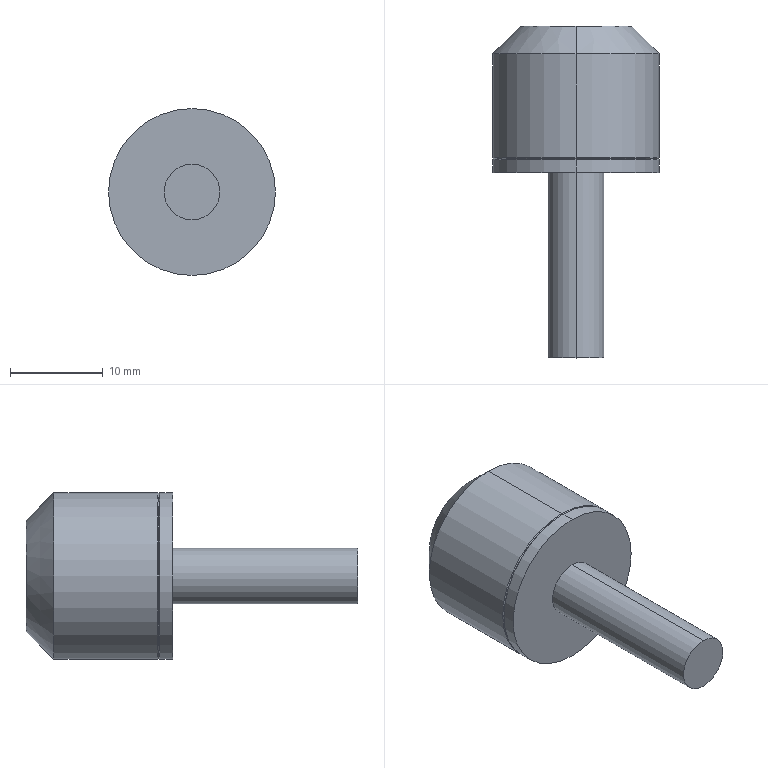Part | STEP file | 1 solid | 15 faces | box 18 x 35.8 x 18 mm | volume 4359 mm3 | cone 6 | cylinder 6 | plane 3 | commonest cylinder face diameters 18 x4 6 x2
STEP:
#1=CARTESIAN_POINT('',(0.,0.,0.));
#2=DIRECTION('',(0.,0.,1.));
#3=DIRECTION('',(1.,0.,0.));
#4=AXIS2_PLACEMENT_3D('',#1,#2,#3);
#5=CARTESIAN_POINT('',(0.,145.8,6.));
#6=VERTEX_POINT('',#5);
#7=CARTESIAN_POINT('',(0.,145.8,-6.));
#8=VERTEX_POINT('',#7);
#9=CARTESIAN_POINT('',(0.,145.8,0.));
#10=DIRECTION('',(0.,1.,0.));
#11=DIRECTION('',(0.,0.,-1.));
#12=AXIS2_PLACEMENT_3D('',#9,#10,#11);
#13=CIRCLE('',#12,6.);
#14=CARTESIAN_POINT('',(0.,145.8,0.));
#15=DIRECTION('',(0.,-1.,0.));
#16=DIRECTION('',(0.,0.,-1.));
#17=AXIS2_PLACEMENT_3D('',#14,#15,#16);
#18=CONICAL_SURFACE('',#17,6.,0.7854);
#19=CARTESIAN_POINT('',(6.283,0.));
#20=DIRECTION('',(-1.,0.));
#21=VECTOR('',#20,1.);
#22=LINE('',#19,#21);
#23=(GEOMETRIC_REPRESENTATION_CONTEXT(2)PARAMETRIC_REPRESENTATION_CONTEXT()REPRESENTATION_CONTEXT('',''));
#24=DEFINITIONAL_REPRESENTATION('',(#22),#23);
#25=PCURVE('',#18,#24);
#26=CARTESIAN_POINT('',(-6.072,145.8,6.072));
#27=DIRECTION('',(0.,-1.,0.));
#28=DIRECTION('',(0.,0.,-1.));
#29=AXIS2_PLACEMENT_3D('',#26,#27,#28);
#30=PLANE('',#29);
#31=CARTESIAN_POINT('',(12.072,6.072));
#32=CARTESIAN_POINT('',(12.072,-4.32));
#33=CARTESIAN_POINT('',(3.072,0.8758));
#34=CARTESIAN_POINT('',(-5.928,6.072));
#35=CARTESIAN_POINT('',(3.072,11.268));
#36=CARTESIAN_POINT('',(12.072,16.464));
#37=CARTESIAN_POINT('',(12.072,6.072));
#38=(BOUNDED_CURVE()B_SPLINE_CURVE(2,(#31,#32,#33,#34,#35,#36,#37),.UNSPECIFIED.,.T.,.F.)B_SPLINE_CURVE_WITH_KNOTS((1,2,2,2,2,1),(-2.094,0.,2.094,4.189,6.283,8.378),.UNSPECIFIED.)CURVE()GEOMETRIC_REPRESENTATION_ITEM()RATIONAL_B_SPLINE_CURVE((1.,0.5,1.,0.5,1.,0.5,1.))REPRESENTATION_ITEM(''));
#39=(GEOMETRIC_REPRESENTATION_CONTEXT(2)PARAMETRIC_REPRESENTATION_CONTEXT()REPRESENTATION_CONTEXT('',''));
#40=DEFINITIONAL_REPRESENTATION('',(#38),#39);
#41=PCURVE('',#30,#40);
#42=SURFACE_CURVE('',#13,(#25,#41),.PCURVE_S1.);
#43=EDGE_CURVE('',#6,#8,#42,.T.);
#44=ORIENTED_EDGE('',*,*,#43,.F.);
#45=CARTESIAN_POINT('',(0.,142.8,9.));
#46=VERTEX_POINT('',#45);
#47=CARTESIAN_POINT('',(0.,145.8,6.));
#48=DIRECTION('',(0.,-0.7071,0.7071));
#49=VECTOR('',#48,1.);
#50=LINE('',#47,#49);
#51=CARTESIAN_POINT('',(3.142,0.));
#52=DIRECTION('',(0.,1.));
#53=VECTOR('',#52,1.);
#54=LINE('',#51,#53);
#55=(GEOMETRIC_REPRESENTATION_CONTEXT(2)PARAMETRIC_REPRESENTATION_CONTEXT()REPRESENTATION_CONTEXT('',''));
#56=DEFINITIONAL_REPRESENTATION('',(#54),#55);
#57=PCURVE('',#18,#56);
#58=CARTESIAN_POINT('',(0.,145.8,0.));
#59=DIRECTION('',(0.,-1.,0.));
#60=DIRECTION('',(0.,0.,-1.));
#61=AXIS2_PLACEMENT_3D('',#58,#59,#60);
#62=CONICAL_SURFACE('',#61,6.,0.7854);
#63=CARTESIAN_POINT('',(3.142,0.));
#64=DIRECTION('',(0.,1.));
#65=VECTOR('',#64,1.);
#66=LINE('',#63,#65);
#67=(GEOMETRIC_REPRESENTATION_CONTEXT(2)PARAMETRIC_REPRESENTATION_CONTEXT()REPRESENTATION_CONTEXT('',''));
#68=DEFINITIONAL_REPRESENTATION('',(#66),#67);
#69=PCURVE('',#62,#68);
#70=SURFACE_CURVE('',#50,(#57,#69),.PCURVE_S1.);
#71=EDGE_CURVE('',#6,#46,#70,.T.);
#72=ORIENTED_EDGE('',*,*,#71,.T.);
#73=CARTESIAN_POINT('',(0.,142.8,-9.));
#74=VERTEX_POINT('',#73);
#75=CARTESIAN_POINT('',(0.,142.8,0.));
#76=DIRECTION('',(0.,-1.,0.));
#77=DIRECTION('',(0.,0.,-1.));
#78=AXIS2_PLACEMENT_3D('',#75,#76,#77);
#79=CIRCLE('',#78,9.);
#80=CARTESIAN_POINT('',(0.,3.));
#81=DIRECTION('',(1.,0.));
#82=VECTOR('',#81,1.);
#83=LINE('',#80,#82);
#84=(GEOMETRIC_REPRESENTATION_CONTEXT(2)PARAMETRIC_REPRESENTATION_CONTEXT()REPRESENTATION_CONTEXT('',''));
#85=DEFINITIONAL_REPRESENTATION('',(#83),#84);
#86=PCURVE('',#18,#85);
#87=CARTESIAN_POINT('',(0.,142.8,0.));
#88=DIRECTION('',(0.,-1.,0.));
#89=DIRECTION('',(0.,0.,-1.));
#90=AXIS2_PLACEMENT_3D('',#87,#88,#89);
#91=CYLINDRICAL_SURFACE('',#90,9.);
#92=CARTESIAN_POINT('',(0.,0.));
#93=DIRECTION('',(1.,0.));
#94=VECTOR('',#93,1.);
#95=LINE('',#92,#94);
#96=(GEOMETRIC_REPRESENTATION_CONTEXT(2)PARAMETRIC_REPRESENTATION_CONTEXT()REPRESENTATION_CONTEXT('',''));
#97=DEFINITIONAL_REPRESENTATION('',(#95),#96);
#98=PCURVE('',#91,#97);
#99=SURFACE_CURVE('',#79,(#86,#98),.PCURVE_S1.);
#100=EDGE_CURVE('',#74,#46,#99,.T.);
#101=ORIENTED_EDGE('',*,*,#100,.F.);
#102=CARTESIAN_POINT('',(0.,145.8,-6.));
#103=DIRECTION('',(0.,-0.7071,-0.7071));
#104=VECTOR('',#103,1.);
#105=LINE('',#102,#104);
#106=CARTESIAN_POINT('',(0.,0.));
#107=DIRECTION('',(0.,1.));
#108=VECTOR('',#107,1.);
#109=LINE('',#106,#108);
#110=(GEOMETRIC_REPRESENTATION_CONTEXT(2)PARAMETRIC_REPRESENTATION_CONTEXT()REPRESENTATION_CONTEXT('',''));
#111=DEFINITIONAL_REPRESENTATION('',(#109),#110);
#112=PCURVE('',#18,#111);
#113=CARTESIAN_POINT('',(6.283,0.));
#114=DIRECTION('',(0.,1.));
#115=VECTOR('',#114,1.);
#116=LINE('',#113,#115);
#117=(GEOMETRIC_REPRESENTATION_CONTEXT(2)PARAMETRIC_REPRESENTATION_CONTEXT()REPRESENTATION_CONTEXT('',''));
#118=DEFINITIONAL_REPRESENTATION('',(#116),#117);
#119=PCURVE('',#62,#118);
#120=SURFACE_CURVE('',#105,(#112,#119),.PCURVE_S1.);
#121=EDGE_CURVE('',#8,#74,#120,.T.);
#122=ORIENTED_EDGE('',*,*,#121,.F.);
#123=EDGE_LOOP('',(#44,#72,#101,#122));
#124=FACE_BOUND('',#123,.T.);
#125=ADVANCED_FACE('',(#124),#18,.T.);
#126=ORIENTED_EDGE('',*,*,#100,.T.);
#127=CARTESIAN_POINT('',(0.,131.6,9.));
#128=VERTEX_POINT('',#127);
#129=CARTESIAN_POINT('',(0.,142.8,9.));
#130=DIRECTION('',(0.,-1.,0.));
#131=VECTOR('',#130,1.);
#132=LINE('',#129,#131);
#133=CARTESIAN_POINT('',(3.142,0.));
#134=DIRECTION('',(0.,1.));
#135=VECTOR('',#134,1.);
#136=LINE('',#133,#135);
#137=(GEOMETRIC_REPRESENTATION_CONTEXT(2)PARAMETRIC_REPRESENTATION_CONTEXT()REPRESENTATION_CONTEXT('',''));
#138=DEFINITIONAL_REPRESENTATION('',(#136),#137);
#139=PCURVE('',#91,#138);
#140=CARTESIAN_POINT('',(0.,142.8,0.));
#141=DIRECTION('',(0.,-1.,0.));
#142=DIRECTION('',(0.,0.,-1.));
#143=AXIS2_PLACEMENT_3D('',#140,#141,#142);
#144=CYLINDRICAL_SURFACE('',#143,9.);
#145=CARTESIAN_POINT('',(3.142,0.));
#146=DIRECTION('',(0.,1.));
#147=VECTOR('',#146,1.);
#148=LINE('',#145,#147);
#149=(GEOMETRIC_REPRESENTATION_CONTEXT(2)PARAMETRIC_REPRESENTATION_CONTEXT()REPRESENTATION_CONTEXT('',''));
#150=DEFINITIONAL_REPRESENTATION('',(#148),#149);
#151=PCURVE('',#144,#150);
#152=SURFACE_CURVE('',#132,(#139,#151),.PCURVE_S1.);
#153=EDGE_CURVE('',#46,#128,#152,.T.);
#154=ORIENTED_EDGE('',*,*,#153,.T.);
#155=CARTESIAN_POINT('',(0.,131.6,-9.));
#156=VERTEX_POINT('',#155);
#157=CARTESIAN_POINT('',(0.,131.6,0.));
#158=DIRECTION('',(0.,-1.,0.));
#159=DIRECTION('',(0.,0.,-1.));
#160=AXIS2_PLACEMENT_3D('',#157,#158,#159);
#161=CIRCLE('',#160,9.);
#162=CARTESIAN_POINT('',(0.,11.2));
#163=DIRECTION('',(1.,0.));
#164=VECTOR('',#163,1.);
#165=LINE('',#162,#164);
#166=(GEOMETRIC_REPRESENTATION_CONTEXT(2)PARAMETRIC_REPRESENTATION_CONTEXT()REPRESENTATION_CONTEXT('',''));
#167=DEFINITIONAL_REPRESENTATION('',(#165),#166);
#168=PCURVE('',#91,#167);
#169=CARTESIAN_POINT('',(0.,131.5,0.));
#170=DIRECTION('',(0.,1.,0.));
#171=DIRECTION('',(0.,0.,1.));
#172=AXIS2_PLACEMENT_3D('',#169,#170,#171);
#173=CONICAL_SURFACE('',#172,8.9,0.7854);
#174=CARTESIAN_POINT('',(3.142,0.1));
#175=DIRECTION('',(-1.,0.));
#176=VECTOR('',#175,1.);
#177=LINE('',#174,#176);
#178=(GEOMETRIC_REPRESENTATION_CONTEXT(2)PARAMETRIC_REPRESENTATION_CONTEXT()REPRESENTATION_CONTEXT('',''));
#179=DEFINITIONAL_REPRESENTATION('',(#177),#178);
#180=PCURVE('',#173,#179);
#181=SURFACE_CURVE('',#161,(#168,#180),.PCURVE_S1.);
#182=EDGE_CURVE('',#156,#128,#181,.T.);
#183=ORIENTED_EDGE('',*,*,#182,.F.);
#184=CARTESIAN_POINT('',(0.,142.8,-9.));
#185=DIRECTION('',(0.,-1.,0.));
#186=VECTOR('',#185,1.);
#187=LINE('',#184,#186);
#188=CARTESIAN_POINT('',(0.,0.));
#189=DIRECTION('',(0.,1.));
#190=VECTOR('',#189,1.);
#191=LINE('',#188,#190);
#192=(GEOMETRIC_REPRESENTATION_CONTEXT(2)PARAMETRIC_REPRESENTATION_CONTEXT()REPRESENTATION_CONTEXT('',''));
#193=DEFINITIONAL_REPRESENTATION('',(#191),#192);
#194=PCURVE('',#91,#193);
#195=CARTESIAN_POINT('',(6.283,0.));
#196=DIRECTION('',(0.,1.));
#197=VECTOR('',#196,1.);
#198=LINE('',#195,#197);
#199=(GEOMETRIC_REPRESENTATION_CONTEXT(2)PARAMETRIC_REPRESENTATION_CONTEXT()REPRESENTATION_CONTEXT('',''));
#200=DEFINITIONAL_REPRESENTATION('',(#198),#199);
#201=PCURVE('',#144,#200);
#202=SURFACE_CURVE('',#187,(#194,#201),.PCURVE_S1.);
#203=EDGE_CURVE('',#74,#156,#202,.T.);
#204=ORIENTED_EDGE('',*,*,#203,.F.);
#205=EDGE_LOOP('',(#126,#154,#183,#204));
#206=FACE_BOUND('',#205,.T.);
#207=ADVANCED_FACE('',(#206),#91,.T.);
#208=CARTESIAN_POINT('',(0.,131.5,-8.9));
#209=VERTEX_POINT('',#208);
#210=CARTESIAN_POINT('',(0.,131.5,8.9));
#211=VERTEX_POINT('',#210);
#212=CARTESIAN_POINT('',(0.,131.5,0.));
#213=DIRECTION('',(0.,-1.,0.));
#214=DIRECTION('',(0.,0.,1.));
#215=AXIS2_PLACEMENT_3D('',#212,#213,#214);
#216=CIRCLE('',#215,8.9);
#217=CARTESIAN_POINT('',(6.283,0.));
#218=DIRECTION('',(-1.,0.));
#219=VECTOR('',#218,1.);
#220=LINE('',#217,#219);
#221=(GEOMETRIC_REPRESENTATION_CONTEXT(2)PARAMETRIC_REPRESENTATION_CONTEXT()REPRESENTATION_CONTEXT('',''));
#222=DEFINITIONAL_REPRESENTATION('',(#220),#221);
#223=PCURVE('',#173,#222);
#224=CARTESIAN_POINT('',(0.,131.5,0.));
#225=DIRECTION('',(0.,-1.,0.));
#226=DIRECTION('',(0.,0.,-1.));
#227=AXIS2_PLACEMENT_3D('',#224,#225,#226);
#228=CONICAL_SURFACE('',#227,8.9,0.7854);
#229=CARTESIAN_POINT('',(-3.142,0.));
#230=DIRECTION('',(1.,0.));
#231=VECTOR('',#230,1.);
#232=LINE('',#229,#231);
#233=(GEOMETRIC_REPRESENTATION_CONTEXT(2)PARAMETRIC_REPRESENTATION_CONTEXT()REPRESENTATION_CONTEXT('',''));
#234=DEFINITIONAL_REPRESENTATION('',(#232),#233);
#235=PCURVE('',#228,#234);
#236=SURFACE_CURVE('',#216,(#223,#235),.PCURVE_S1.);
#237=EDGE_CURVE('',#209,#211,#236,.T.);
#238=ORIENTED_EDGE('',*,*,#237,.F.);
#239=CARTESIAN_POINT('',(0.,131.5,-8.9));
#240=DIRECTION('',(0.,0.7071,-0.7071));
#241=VECTOR('',#240,1.);
#242=LINE('',#239,#241);
#243=CARTESIAN_POINT('',(3.142,0.));
#244=DIRECTION('',(0.,1.));
#245=VECTOR('',#244,1.);
#246=LINE('',#243,#245);
#247=(GEOMETRIC_REPRESENTATION_CONTEXT(2)PARAMETRIC_REPRESENTATION_CONTEXT()REPRESENTATION_CONTEXT('',''));
#248=DEFINITIONAL_REPRESENTATION('',(#246),#247);
#249=PCURVE('',#173,#248);
#250=CARTESIAN_POINT('',(0.,131.5,0.));
#251=DIRECTION('',(0.,1.,0.));
#252=DIRECTION('',(0.,0.,1.));
#253=AXIS2_PLACEMENT_3D('',#250,#251,#252);
#254=CONICAL_SURFACE('',#253,8.9,0.7854);
#255=CARTESIAN_POINT('',(3.142,0.));
#256=DIRECTION('',(0.,1.));
#257=VECTOR('',#256,1.);
#258=LINE('',#255,#257);
#259=(GEOMETRIC_REPRESENTATION_CONTEXT(2)PARAMETRIC_REPRESENTATION_CONTEXT()REPRESENTATION_CONTEXT('',''));
#260=DEFINITIONAL_REPRESENTATION('',(#258),#259);
#261=PCURVE('',#254,#260);
#262=SURFACE_CURVE('',#242,(#249,#261),.PCURVE_S1.);
#263=EDGE_CURVE('',#209,#156,#262,.T.);
#264=ORIENTED_EDGE('',*,*,#263,.T.);
#265=ORIENTED_EDGE('',*,*,#182,.T.);
#266=CARTESIAN_POINT('',(0.,131.5,8.9));
#267=DIRECTION('',(0.,0.7071,0.7071));
#268=VECTOR('',#267,1.);
#269=LINE('',#266,#268);
#270=CARTESIAN_POINT('',(0.,0.));
#271=DIRECTION('',(0.,1.));
#272=VECTOR('',#271,1.);
#273=LINE('',#270,#272);
#274=(GEOMETRIC_REPRESENTATION_CONTEXT(2)PARAMETRIC_REPRESENTATION_CONTEXT()REPRESENTATION_CONTEXT('',''));
#275=DEFINITIONAL_REPRESENTATION('',(#273),#274);
#276=PCURVE('',#173,#275);
#277=CARTESIAN_POINT('',(6.283,0.));
#278=DIRECTION('',(0.,1.));
#279=VECTOR('',#278,1.);
#280=LINE('',#277,#279);
#281=(GEOMETRIC_REPRESENTATION_CONTEXT(2)PARAMETRIC_REPRESENTATION_CONTEXT()REPRESENTATION_CONTEXT('',''));
#282=DEFINITIONAL_REPRESENTATION('',(#280),#281);
#283=PCURVE('',#254,#282);
#284=SURFACE_CURVE('',#269,(#276,#283),.PCURVE_S1.);
#285=EDGE_CURVE('',#211,#128,#284,.T.);
#286=ORIENTED_EDGE('',*,*,#285,.F.);
#287=EDGE_LOOP('',(#238,#264,#265,#286));
#288=FACE_BOUND('',#287,.T.);
#289=ADVANCED_FACE('',(#288),#173,.T.);
#290=ORIENTED_EDGE('',*,*,#237,.T.);
#291=CARTESIAN_POINT('',(0.,131.4,9.));
#292=VERTEX_POINT('',#291);
#293=CARTESIAN_POINT('',(0.,131.5,8.9));
#294=DIRECTION('',(0.,-0.7071,0.7071));
#295=VECTOR('',#294,1.);
#296=LINE('',#293,#295);
#297=CARTESIAN_POINT('',(3.142,0.));
#298=DIRECTION('',(0.,1.));
#299=VECTOR('',#298,1.);
#300=LINE('',#297,#299);
#301=(GEOMETRIC_REPRESENTATION_CONTEXT(2)PARAMETRIC_REPRESENTATION_CONTEXT()REPRESENTATION_CONTEXT('',''));
#302=DEFINITIONAL_REPRESENTATION('',(#300),#301);
#303=PCURVE('',#228,#302);
#304=CARTESIAN_POINT('',(0.,131.5,0.));
#305=DIRECTION('',(0.,-1.,0.));
#306=DIRECTION('',(0.,0.,-1.));
#307=AXIS2_PLACEMENT_3D('',#304,#305,#306);
#308=CONICAL_SURFACE('',#307,8.9,0.7854);
#309=CARTESIAN_POINT('',(3.142,0.));
#310=DIRECTION('',(0.,1.));
#311=VECTOR('',#310,1.);
#312=LINE('',#309,#311);
#313=(GEOMETRIC_REPRESENTATION_CONTEXT(2)PARAMETRIC_REPRESENTATION_CONTEXT()REPRESENTATION_CONTEXT('',''));
#314=DEFINITIONAL_REPRESENTATION('',(#312),#313);
#315=PCURVE('',#308,#314);
#316=SURFACE_CURVE('',#296,(#303,#315),.PCURVE_S1.);
#317=EDGE_CURVE('',#211,#292,#316,.T.);
#318=ORIENTED_EDGE('',*,*,#317,.T.);
#319=CARTESIAN_POINT('',(0.,131.4,-9.));
#320=VERTEX_POINT('',#319);
#321=CARTESIAN_POINT('',(0.,131.4,0.));
#322=DIRECTION('',(0.,-1.,0.));
#323=DIRECTION('',(0.,0.,-1.));
#324=AXIS2_PLACEMENT_3D('',#321,#322,#323);
#325=CIRCLE('',#324,9.);
#326=CARTESIAN_POINT('',(0.,0.1));
#327=DIRECTION('',(1.,0.));
#328=VECTOR('',#327,1.);
#329=LINE('',#326,#328);
#330=(GEOMETRIC_REPRESENTATION_CONTEXT(2)PARAMETRIC_REPRESENTATION_CONTEXT()REPRESENTATION_CONTEXT('',''));
#331=DEFINITIONAL_REPRESENTATION('',(#329),#330);
#332=PCURVE('',#228,#331);
#333=CARTESIAN_POINT('',(0.,131.4,0.));
#334=DIRECTION('',(0.,-1.,0.));
#335=DIRECTION('',(0.,0.,-1.));
#336=AXIS2_PLACEMENT_3D('',#333,#334,#335);
#337=CYLINDRICAL_SURFACE('',#336,9.);
#338=CARTESIAN_POINT('',(0.,0.));
#339=DIRECTION('',(1.,0.));
#340=VECTOR('',#339,1.);
#341=LINE('',#338,#340);
#342=(GEOMETRIC_REPRESENTATION_CONTEXT(2)PARAMETRIC_REPRESENTATION_CONTEXT()REPRESENTATION_CONTEXT('',''));
#343=DEFINITIONAL_REPRESENTATION('',(#341),#342);
#344=PCURVE('',#337,#343);
#345=SURFACE_CURVE('',#325,(#332,#344),.PCURVE_S1.);
#346=EDGE_CURVE('',#320,#292,#345,.T.);
#347=ORIENTED_EDGE('',*,*,#346,.F.);
#348=CARTESIAN_POINT('',(0.,131.5,-8.9));
#349=DIRECTION('',(0.,-0.7071,-0.7071));
#350=VECTOR('',#349,1.);
#351=LINE('',#348,#350);
#352=CARTESIAN_POINT('',(0.,0.));
#353=DIRECTION('',(0.,1.));
#354=VECTOR('',#353,1.);
#355=LINE('',#352,#354);
#356=(GEOMETRIC_REPRESENTATION_CONTEXT(2)PARAMETRIC_REPRESENTATION_CONTEXT()REPRESENTATION_CONTEXT('',''));
#357=DEFINITIONAL_REPRESENTATION('',(#355),#356);
#358=PCURVE('',#228,#357);
#359=CARTESIAN_POINT('',(6.283,0.));
#360=DIRECTION('',(0.,1.));
#361=VECTOR('',#360,1.);
#362=LINE('',#359,#361);
#363=(GEOMETRIC_REPRESENTATION_CONTEXT(2)PARAMETRIC_REPRESENTATION_CONTEXT()REPRESENTATION_CONTEXT('',''));
#364=DEFINITIONAL_REPRESENTATION('',(#362),#363);
#365=PCURVE('',#308,#364);
#366=SURFACE_CURVE('',#351,(#358,#365),.PCURVE_S1.);
#367=EDGE_CURVE('',#209,#320,#366,.T.);
#368=ORIENTED_EDGE('',*,*,#367,.F.);
#369=EDGE_LOOP('',(#290,#318,#347,#368));
#370=FACE_BOUND('',#369,.T.);
#371=ADVANCED_FACE('',(#370),#228,.T.);
#372=ORIENTED_EDGE('',*,*,#346,.T.);
#373=CARTESIAN_POINT('',(0.,130.,9.));
#374=VERTEX_POINT('',#373);
#375=CARTESIAN_POINT('',(0.,131.4,9.));
#376=DIRECTION('',(0.,-1.,0.));
#377=VECTOR('',#376,1.);
#378=LINE('',#375,#377);
#379=CARTESIAN_POINT('',(3.142,0.));
#380=DIRECTION('',(0.,1.));
#381=VECTOR('',#380,1.);
#382=LINE('',#379,#381);
#383=(GEOMETRIC_REPRESENTATION_CONTEXT(2)PARAMETRIC_REPRESENTATION_CONTEXT()REPRESENTATION_CONTEXT('',''));
#384=DEFINITIONAL_REPRESENTATION('',(#382),#383);
#385=PCURVE('',#337,#384);
#386=CARTESIAN_POINT('',(0.,131.4,0.));
#387=DIRECTION('',(0.,-1.,0.));
#388=DIRECTION('',(0.,0.,-1.));
#389=AXIS2_PLACEMENT_3D('',#386,#387,#388);
#390=CYLINDRICAL_SURFACE('',#389,9.);
#391=CARTESIAN_POINT('',(3.142,0.));
#392=DIRECTION('',(0.,1.));
#393=VECTOR('',#392,1.);
#394=LINE('',#391,#393);
#395=(GEOMETRIC_REPRESENTATION_CONTEXT(2)PARAMETRIC_REPRESENTATION_CONTEXT()REPRESENTATION_CONTEXT('',''));
#396=DEFINITIONAL_REPRESENTATION('',(#394),#395);
#397=PCURVE('',#390,#396);
#398=SURFACE_CURVE('',#378,(#385,#397),.PCURVE_S1.);
#399=EDGE_CURVE('',#292,#374,#398,.T.);
#400=ORIENTED_EDGE('',*,*,#399,.T.);
#401=CARTESIAN_POINT('',(0.,130.,-9.));
#402=VERTEX_POINT('',#401);
#403=CARTESIAN_POINT('',(0.,130.,0.));
#404=DIRECTION('',(0.,-1.,0.));
#405=DIRECTION('',(0.,0.,-1.));
#406=AXIS2_PLACEMENT_3D('',#403,#404,#405);
#407=CIRCLE('',#406,9.);
#408=CARTESIAN_POINT('',(0.,1.4));
#409=DIRECTION('',(1.,0.));
#410=VECTOR('',#409,1.);
#411=LINE('',#408,#410);
#412=(GEOMETRIC_REPRESENTATION_CONTEXT(2)PARAMETRIC_REPRESENTATION_CONTEXT()REPRESENTATION_CONTEXT('',''));
#413=DEFINITIONAL_REPRESENTATION('',(#411),#412);
#414=PCURVE('',#337,#413);
#415=CARTESIAN_POINT('',(-9.108,130.,-9.108));
#416=DIRECTION('',(0.,1.,0.));
#417=DIRECTION('',(0.,0.,1.));
#418=AXIS2_PLACEMENT_3D('',#415,#416,#417);
#419=PLANE('',#418);
#420=CARTESIAN_POINT('',(0.108,9.108));
#421=CARTESIAN_POINT('',(0.108,24.696));
#422=CARTESIAN_POINT('',(13.608,16.902));
#423=CARTESIAN_POINT('',(27.108,9.108));
#424=CARTESIAN_POINT('',(13.608,1.314));
#425=CARTESIAN_POINT('',(0.108,-6.48));
#426=CARTESIAN_POINT('',(0.108,9.108));
#427=(BOUNDED_CURVE()B_SPLINE_CURVE(2,(#420,#421,#422,#423,#424,#425,#426),.UNSPECIFIED.,.T.,.F.)B_SPLINE_CURVE_WITH_KNOTS((1,2,2,2,2,1),(-2.094,0.,2.094,4.189,6.283,8.378),.UNSPECIFIED.)CURVE()GEOMETRIC_REPRESENTATION_ITEM()RATIONAL_B_SPLINE_CURVE((1.,0.5,1.,0.5,1.,0.5,1.))REPRESENTATION_ITEM(''));
#428=(GEOMETRIC_REPRESENTATION_CONTEXT(2)PARAMETRIC_REPRESENTATION_CONTEXT()REPRESENTATION_CONTEXT('',''));
#429=DEFINITIONAL_REPRESENTATION('',(#427),#428);
#430=PCURVE('',#419,#429);
#431=SURFACE_CURVE('',#407,(#414,#430),.PCURVE_S1.);
#432=EDGE_CURVE('',#402,#374,#431,.T.);
#433=ORIENTED_EDGE('',*,*,#432,.F.);
#434=CARTESIAN_POINT('',(0.,131.4,-9.));
#435=DIRECTION('',(0.,-1.,0.));
#436=VECTOR('',#435,1.);
#437=LINE('',#434,#436);
#438=CARTESIAN_POINT('',(0.,0.));
#439=DIRECTION('',(0.,1.));
#440=VECTOR('',#439,1.);
#441=LINE('',#438,#440);
#442=(GEOMETRIC_REPRESENTATION_CONTEXT(2)PARAMETRIC_REPRESENTATION_CONTEXT()REPRESENTATION_CONTEXT('',''));
#443=DEFINITIONAL_REPRESENTATION('',(#441),#442);
#444=PCURVE('',#337,#443);
#445=CARTESIAN_POINT('',(6.283,0.));
#446=DIRECTION('',(0.,1.));
#447=VECTOR('',#446,1.);
#448=LINE('',#445,#447);
#449=(GEOMETRIC_REPRESENTATION_CONTEXT(2)PARAMETRIC_REPRESENTATION_CONTEXT()REPRESENTATION_CONTEXT('',''));
#450=DEFINITIONAL_REPRESENTATION('',(#448),#449);
#451=PCURVE('',#390,#450);
#452=SURFACE_CURVE('',#437,(#444,#451),.PCURVE_S1.);
#453=EDGE_CURVE('',#320,#402,#452,.T.);
#454=ORIENTED_EDGE('',*,*,#453,.F.);
#455=EDGE_LOOP('',(#372,#400,#433,#454));
#456=FACE_BOUND('',#455,.T.);
#457=ADVANCED_FACE('',(#456),#337,.T.);
#458=CARTESIAN_POINT('',(0.,130.,-3.));
#459=VERTEX_POINT('',#458);
#460=CARTESIAN_POINT('',(0.,130.,3.));
#461=VERTEX_POINT('',#460);
#462=CARTESIAN_POINT('',(0.,130.,0.));
#463=DIRECTION('',(0.,-1.,0.));
#464=DIRECTION('',(0.,0.,-1.));
#465=AXIS2_PLACEMENT_3D('',#462,#463,#464);
#466=CIRCLE('',#465,3.);
#467=CARTESIAN_POINT('',(0.,130.,0.));
#468=DIRECTION('',(0.,-1.,0.));
#469=DIRECTION('',(0.,0.,-1.));
#470=AXIS2_PLACEMENT_3D('',#467,#468,#469);
#471=CYLINDRICAL_SURFACE('',#470,3.);
#472=CARTESIAN_POINT('',(0.,0.));
#473=DIRECTION('',(1.,0.));
#474=VECTOR('',#473,1.);
#475=LINE('',#472,#474);
#476=(GEOMETRIC_REPRESENTATION_CONTEXT(2)PARAMETRIC_REPRESENTATION_CONTEXT()REPRESENTATION_CONTEXT('',''));
#477=DEFINITIONAL_REPRESENTATION('',(#475),#476);
#478=PCURVE('',#471,#477);
#479=CARTESIAN_POINT('',(6.108,9.108));
#480=CARTESIAN_POINT('',(6.108,14.304));
#481=CARTESIAN_POINT('',(10.608,11.706));
#482=CARTESIAN_POINT('',(15.108,9.108));
#483=CARTESIAN_POINT('',(10.608,6.51));
#484=CARTESIAN_POINT('',(6.108,3.912));
#485=CARTESIAN_POINT('',(6.108,9.108));
#486=(BOUNDED_CURVE()B_SPLINE_CURVE(2,(#479,#480,#481,#482,#483,#484,#485),.UNSPECIFIED.,.T.,.F.)B_SPLINE_CURVE_WITH_KNOTS((1,2,2,2,2,1),(-2.094,0.,2.094,4.189,6.283,8.378),.UNSPECIFIED.)CURVE()GEOMETRIC_REPRESENTATION_ITEM()RATIONAL_B_SPLINE_CURVE((1.,0.5,1.,0.5,1.,0.5,1.))REPRESENTATION_ITEM(''));
#487=(GEOMETRIC_REPRESENTATION_CONTEXT(2)PARAMETRIC_REPRESENTATION_CONTEXT()REPRESENTATION_CONTEXT('',''));
#488=DEFINITIONAL_REPRESENTATION('',(#486),#487);
#489=PCURVE('',#419,#488);
#490=SURFACE_CURVE('',#466,(#478,#489),.PCURVE_S1.);
#491=EDGE_CURVE('',#459,#461,#490,.T.);
#492=ORIENTED_EDGE('',*,*,#491,.T.);
#493=CARTESIAN_POINT('',(0.,110.,3.));
#494=VERTEX_POINT('',#493);
#495=CARTESIAN_POINT('',(0.,130.,3.));
#496=DIRECTION('',(0.,-1.,0.));
#497=VECTOR('',#496,1.);
#498=LINE('',#495,#497);
#499=CARTESIAN_POINT('',(3.142,0.));
#500=DIRECTION('',(0.,1.));
#501=VECTOR('',#500,1.);
#502=LINE('',#499,#501);
#503=(GEOMETRIC_REPRESENTATION_CONTEXT(2)PARAMETRIC_REPRESENTATION_CONTEXT()REPRESENTATION_CONTEXT('',''));
#504=DEFINITIONAL_REPRESENTATION('',(#502),#503);
#505=PCURVE('',#471,#504);
#506=CARTESIAN_POINT('',(0.,130.,0.));
#507=DIRECTION('',(0.,-1.,0.));
#508=DIRECTION('',(0.,0.,-1.));
#509=AXIS2_PLACEMENT_3D('',#506,#507,#508);
#510=CYLINDRICAL_SURFACE('',#509,3.);
#511=CARTESIAN_POINT('',(3.142,0.));
#512=DIRECTION('',(0.,1.));
#513=VECTOR('',#512,1.);
#514=LINE('',#511,#513);
#515=(GEOMETRIC_REPRESENTATION_CONTEXT(2)PARAMETRIC_REPRESENTATION_CONTEXT()REPRESENTATION_CONTEXT('',''));
#516=DEFINITIONAL_REPRESENTATION('',(#514),#515);
#517=PCURVE('',#510,#516);
#518=SURFACE_CURVE('',#498,(#505,#517),.PCURVE_S1.);
#519=EDGE_CURVE('',#461,#494,#518,.T.);
#520=ORIENTED_EDGE('',*,*,#519,.T.);
#521=CARTESIAN_POINT('',(0.,110.,-3.));
#522=VERTEX_POINT('',#521);
#523=CARTESIAN_POINT('',(0.,110.,0.));
#524=DIRECTION('',(0.,-1.,0.));
#525=DIRECTION('',(0.,0.,-1.));
#526=AXIS2_PLACEMENT_3D('',#523,#524,#525);
#527=CIRCLE('',#526,3.);
#528=CARTESIAN_POINT('',(0.,20.));
#529=DIRECTION('',(1.,0.));
#530=VECTOR('',#529,1.);
#531=LINE('',#528,#530);
#532=(GEOMETRIC_REPRESENTATION_CONTEXT(2)PARAMETRIC_REPRESENTATION_CONTEXT()REPRESENTATION_CONTEXT('',''));
#533=DEFINITIONAL_REPRESENTATION('',(#531),#532);
#534=PCURVE('',#471,#533);
#535=CARTESIAN_POINT('',(-3.036,110.,-3.036));
#536=DIRECTION('',(0.,1.,0.));
#537=DIRECTION('',(0.,0.,1.));
#538=AXIS2_PLACEMENT_3D('',#535,#536,#537);
#539=PLANE('',#538);
#540=CARTESIAN_POINT('',(0.036,3.036));
#541=CARTESIAN_POINT('',(0.036,8.232));
#542=CARTESIAN_POINT('',(4.536,5.634));
#543=CARTESIAN_POINT('',(9.036,3.036));
#544=CARTESIAN_POINT('',(4.536,0.4379));
#545=CARTESIAN_POINT('',(0.036,-2.16));
#546=CARTESIAN_POINT('',(0.036,3.036));
#547=(BOUNDED_CURVE()B_SPLINE_CURVE(2,(#540,#541,#542,#543,#544,#545,#546),.UNSPECIFIED.,.T.,.F.)B_SPLINE_CURVE_WITH_KNOTS((1,2,2,2,2,1),(-2.094,0.,2.094,4.189,6.283,8.378),.UNSPECIFIED.)CURVE()GEOMETRIC_REPRESENTATION_ITEM()RATIONAL_B_SPLINE_CURVE((1.,0.5,1.,0.5,1.,0.5,1.))REPRESENTATION_ITEM(''));
#548=(GEOMETRIC_REPRESENTATION_CONTEXT(2)PARAMETRIC_REPRESENTATION_CONTEXT()REPRESENTATION_CONTEXT('',''));
#549=DEFINITIONAL_REPRESENTATION('',(#547),#548);
#550=PCURVE('',#539,#549);
#551=SURFACE_CURVE('',#527,(#534,#550),.PCURVE_S1.);
#552=EDGE_CURVE('',#522,#494,#551,.T.);
#553=ORIENTED_EDGE('',*,*,#552,.F.);
#554=CARTESIAN_POINT('',(0.,130.,-3.));
#555=DIRECTION('',(0.,-1.,0.));
#556=VECTOR('',#555,1.);
#557=LINE('',#554,#556);
#558=CARTESIAN_POINT('',(0.,0.));
#559=DIRECTION('',(0.,1.));
#560=VECTOR('',#559,1.);
#561=LINE('',#558,#560);
#562=(GEOMETRIC_REPRESENTATION_CONTEXT(2)PARAMETRIC_REPRESENTATION_CONTEXT()REPRESENTATION_CONTEXT('',''));
#563=DEFINITIONAL_REPRESENTATION('',(#561),#562);
#564=PCURVE('',#471,#563);
#565=CARTESIAN_POINT('',(6.283,0.));
#566=DIRECTION('',(0.,1.));
#567=VECTOR('',#566,1.);
#568=LINE('',#565,#567);
#569=(GEOMETRIC_REPRESENTATION_CONTEXT(2)PARAMETRIC_REPRESENTATION_CONTEXT()REPRESENTATION_CONTEXT('',''));
#570=DEFINITIONAL_REPRESENTATION('',(#568),#569);
#571=PCURVE('',#510,#570);
#572=SURFACE_CURVE('',#557,(#564,#571),.PCURVE_S1.);
#573=EDGE_CURVE('',#459,#522,#572,.T.);
#574=ORIENTED_EDGE('',*,*,#573,.F.);
#575=EDGE_LOOP('',(#492,#520,#553,#574));
#576=FACE_BOUND('',#575,.T.);
#577=ADVANCED_FACE('',(#576),#471,.T.);
#578=ORIENTED_EDGE('',*,*,#71,.F.);
#579=CARTESIAN_POINT('',(0.,145.8,0.));
#580=DIRECTION('',(0.,1.,0.));
#581=DIRECTION('',(0.,0.,-1.));
#582=AXIS2_PLACEMENT_3D('',#579,#580,#581);
#583=CIRCLE('',#582,6.);
#584=CARTESIAN_POINT('',(6.283,0.));
#585=DIRECTION('',(-1.,0.));
#586=VECTOR('',#585,1.);
#587=LINE('',#584,#586);
#588=(GEOMETRIC_REPRESENTATION_CONTEXT(2)PARAMETRIC_REPRESENTATION_CONTEXT()REPRESENTATION_CONTEXT('',''));
#589=DEFINITIONAL_REPRESENTATION('',(#587),#588);
#590=PCURVE('',#62,#589);
#591=CARTESIAN_POINT('',(12.072,6.072));
#592=CARTESIAN_POINT('',(12.072,-4.32));
#593=CARTESIAN_POINT('',(3.072,0.8758));
#594=CARTESIAN_POINT('',(-5.928,6.072));
#595=CARTESIAN_POINT('',(3.072,11.268));
#596=CARTESIAN_POINT('',(12.072,16.464));
#597=CARTESIAN_POINT('',(12.072,6.072));
#598=(BOUNDED_CURVE()B_SPLINE_CURVE(2,(#591,#592,#593,#594,#595,#596,#597),.UNSPECIFIED.,.T.,.F.)B_SPLINE_CURVE_WITH_KNOTS((1,2,2,2,2,1),(-2.094,0.,2.094,4.189,6.283,8.378),.UNSPECIFIED.)CURVE()GEOMETRIC_REPRESENTATION_ITEM()RATIONAL_B_SPLINE_CURVE((1.,0.5,1.,0.5,1.,0.5,1.))REPRESENTATION_ITEM(''));
#599=(GEOMETRIC_REPRESENTATION_CONTEXT(2)PARAMETRIC_REPRESENTATION_CONTEXT()REPRESENTATION_CONTEXT('',''));
#600=DEFINITIONAL_REPRESENTATION('',(#598),#599);
#601=PCURVE('',#30,#600);
#602=SURFACE_CURVE('',#583,(#590,#601),.PCURVE_S1.);
#603=EDGE_CURVE('',#8,#6,#602,.T.);
#604=ORIENTED_EDGE('',*,*,#603,.F.);
#605=ORIENTED_EDGE('',*,*,#121,.T.);
#606=CARTESIAN_POINT('',(0.,142.8,0.));
#607=DIRECTION('',(0.,-1.,0.));
#608=DIRECTION('',(0.,0.,-1.));
#609=AXIS2_PLACEMENT_3D('',#606,#607,#608);
#610=CIRCLE('',#609,9.);
#611=CARTESIAN_POINT('',(0.,3.));
#612=DIRECTION('',(1.,0.));
#613=VECTOR('',#612,1.);
#614=LINE('',#611,#613);
#615=(GEOMETRIC_REPRESENTATION_CONTEXT(2)PARAMETRIC_REPRESENTATION_CONTEXT()REPRESENTATION_CONTEXT('',''));
#616=DEFINITIONAL_REPRESENTATION('',(#614),#615);
#617=PCURVE('',#62,#616);
#618=CARTESIAN_POINT('',(0.,0.));
#619=DIRECTION('',(1.,0.));
#620=VECTOR('',#619,1.);
#621=LINE('',#618,#620);
#622=(GEOMETRIC_REPRESENTATION_CONTEXT(2)PARAMETRIC_REPRESENTATION_CONTEXT()REPRESENTATION_CONTEXT('',''));
#623=DEFINITIONAL_REPRESENTATION('',(#621),#622);
#624=PCURVE('',#144,#623);
#625=SURFACE_CURVE('',#610,(#617,#624),.PCURVE_S1.);
#626=EDGE_CURVE('',#46,#74,#625,.T.);
#627=ORIENTED_EDGE('',*,*,#626,.F.);
#628=EDGE_LOOP('',(#578,#604,#605,#627));
#629=FACE_BOUND('',#628,.T.);
#630=ADVANCED_FACE('',(#629),#62,.T.);
#631=ORIENTED_EDGE('',*,*,#603,.T.);
#632=ORIENTED_EDGE('',*,*,#43,.T.);
#633=EDGE_LOOP('',(#631,#632));
#634=FACE_BOUND('',#633,.T.);
#635=ADVANCED_FACE('',(#634),#30,.F.);
#636=ORIENTED_EDGE('',*,*,#153,.F.);
#637=ORIENTED_EDGE('',*,*,#626,.T.);
#638=ORIENTED_EDGE('',*,*,#203,.T.);
#639=CARTESIAN_POINT('',(0.,131.6,0.));
#640=DIRECTION('',(0.,-1.,0.));
#641=DIRECTION('',(0.,0.,-1.));
#642=AXIS2_PLACEMENT_3D('',#639,#640,#641);
#643=CIRCLE('',#642,9.);
#644=CARTESIAN_POINT('',(0.,11.2));
#645=DIRECTION('',(1.,0.));
#646=VECTOR('',#645,1.);
#647=LINE('',#644,#646);
#648=(GEOMETRIC_REPRESENTATION_CONTEXT(2)PARAMETRIC_REPRESENTATION_CONTEXT()REPRESENTATION_CONTEXT('',''));
#649=DEFINITIONAL_REPRESENTATION('',(#647),#648);
#650=PCURVE('',#144,#649);
#651=CARTESIAN_POINT('',(9.425,0.1));
#652=DIRECTION('',(-1.,0.));
#653=VECTOR('',#652,1.);
#654=LINE('',#651,#653);
#655=(GEOMETRIC_REPRESENTATION_CONTEXT(2)PARAMETRIC_REPRESENTATION_CONTEXT()REPRESENTATION_CONTEXT('',''));
#656=DEFINITIONAL_REPRESENTATION('',(#654),#655);
#657=PCURVE('',#254,#656);
#658=SURFACE_CURVE('',#643,(#650,#657),.PCURVE_S1.);
#659=EDGE_CURVE('',#128,#156,#658,.T.);
#660=ORIENTED_EDGE('',*,*,#659,.F.);
#661=EDGE_LOOP('',(#636,#637,#638,#660));
#662=FACE_BOUND('',#661,.T.);
#663=ADVANCED_FACE('',(#662),#144,.T.);
#664=ORIENTED_EDGE('',*,*,#263,.F.);
#665=CARTESIAN_POINT('',(0.,131.5,0.));
#666=DIRECTION('',(0.,-1.,0.));
#667=DIRECTION('',(0.,0.,1.));
#668=AXIS2_PLACEMENT_3D('',#665,#666,#667);
#669=CIRCLE('',#668,8.9);
#670=CARTESIAN_POINT('',(6.283,0.));
#671=DIRECTION('',(-1.,0.));
#672=VECTOR('',#671,1.);
#673=LINE('',#670,#672);
#674=(GEOMETRIC_REPRESENTATION_CONTEXT(2)PARAMETRIC_REPRESENTATION_CONTEXT()REPRESENTATION_CONTEXT('',''));
#675=DEFINITIONAL_REPRESENTATION('',(#673),#674);
#676=PCURVE('',#254,#675);
#677=CARTESIAN_POINT('',(3.142,0.));
#678=DIRECTION('',(1.,0.));
#679=VECTOR('',#678,1.);
#680=LINE('',#677,#679);
#681=(GEOMETRIC_REPRESENTATION_CONTEXT(2)PARAMETRIC_REPRESENTATION_CONTEXT()REPRESENTATION_CONTEXT('',''));
#682=DEFINITIONAL_REPRESENTATION('',(#680),#681);
#683=PCURVE('',#308,#682);
#684=SURFACE_CURVE('',#669,(#676,#683),.PCURVE_S1.);
#685=EDGE_CURVE('',#211,#209,#684,.T.);
#686=ORIENTED_EDGE('',*,*,#685,.F.);
#687=ORIENTED_EDGE('',*,*,#285,.T.);
#688=ORIENTED_EDGE('',*,*,#659,.T.);
#689=EDGE_LOOP('',(#664,#686,#687,#688));
#690=FACE_BOUND('',#689,.T.);
#691=ADVANCED_FACE('',(#690),#254,.T.);
#692=ORIENTED_EDGE('',*,*,#317,.F.);
#693=ORIENTED_EDGE('',*,*,#685,.T.);
#694=ORIENTED_EDGE('',*,*,#367,.T.);
#695=CARTESIAN_POINT('',(0.,131.4,0.));
#696=DIRECTION('',(0.,-1.,0.));
#697=DIRECTION('',(0.,0.,-1.));
#698=AXIS2_PLACEMENT_3D('',#695,#696,#697);
#699=CIRCLE('',#698,9.);
#700=CARTESIAN_POINT('',(0.,0.1));
#701=DIRECTION('',(1.,0.));
#702=VECTOR('',#701,1.);
#703=LINE('',#700,#702);
#704=(GEOMETRIC_REPRESENTATION_CONTEXT(2)PARAMETRIC_REPRESENTATION_CONTEXT()REPRESENTATION_CONTEXT('',''));
#705=DEFINITIONAL_REPRESENTATION('',(#703),#704);
#706=PCURVE('',#308,#705);
#707=CARTESIAN_POINT('',(0.,0.));
#708=DIRECTION('',(1.,0.));
#709=VECTOR('',#708,1.);
#710=LINE('',#707,#709);
#711=(GEOMETRIC_REPRESENTATION_CONTEXT(2)PARAMETRIC_REPRESENTATION_CONTEXT()REPRESENTATION_CONTEXT('',''));
#712=DEFINITIONAL_REPRESENTATION('',(#710),#711);
#713=PCURVE('',#390,#712);
#714=SURFACE_CURVE('',#699,(#706,#713),.PCURVE_S1.);
#715=EDGE_CURVE('',#292,#320,#714,.T.);
#716=ORIENTED_EDGE('',*,*,#715,.F.);
#717=EDGE_LOOP('',(#692,#693,#694,#716));
#718=FACE_BOUND('',#717,.T.);
#719=ADVANCED_FACE('',(#718),#308,.T.);
#720=ORIENTED_EDGE('',*,*,#399,.F.);
#721=ORIENTED_EDGE('',*,*,#715,.T.);
#722=ORIENTED_EDGE('',*,*,#453,.T.);
#723=CARTESIAN_POINT('',(0.,130.,0.));
#724=DIRECTION('',(0.,-1.,0.));
#725=DIRECTION('',(0.,0.,-1.));
#726=AXIS2_PLACEMENT_3D('',#723,#724,#725);
#727=CIRCLE('',#726,9.);
#728=CARTESIAN_POINT('',(0.,1.4));
#729=DIRECTION('',(1.,0.));
#730=VECTOR('',#729,1.);
#731=LINE('',#728,#730);
#732=(GEOMETRIC_REPRESENTATION_CONTEXT(2)PARAMETRIC_REPRESENTATION_CONTEXT()REPRESENTATION_CONTEXT('',''));
#733=DEFINITIONAL_REPRESENTATION('',(#731),#732);
#734=PCURVE('',#390,#733);
#735=CARTESIAN_POINT('',(0.108,9.108));
#736=CARTESIAN_POINT('',(0.108,24.696));
#737=CARTESIAN_POINT('',(13.608,16.902));
#738=CARTESIAN_POINT('',(27.108,9.108));
#739=CARTESIAN_POINT('',(13.608,1.314));
#740=CARTESIAN_POINT('',(0.108,-6.48));
#741=CARTESIAN_POINT('',(0.108,9.108));
#742=(BOUNDED_CURVE()B_SPLINE_CURVE(2,(#735,#736,#737,#738,#739,#740,#741),.UNSPECIFIED.,.T.,.F.)B_SPLINE_CURVE_WITH_KNOTS((1,2,2,2,2,1),(-2.094,0.,2.094,4.189,6.283,8.378),.UNSPECIFIED.)CURVE()GEOMETRIC_REPRESENTATION_ITEM()RATIONAL_B_SPLINE_CURVE((1.,0.5,1.,0.5,1.,0.5,1.))REPRESENTATION_ITEM(''));
#743=(GEOMETRIC_REPRESENTATION_CONTEXT(2)PARAMETRIC_REPRESENTATION_CONTEXT()REPRESENTATION_CONTEXT('',''));
#744=DEFINITIONAL_REPRESENTATION('',(#742),#743);
#745=PCURVE('',#419,#744);
#746=SURFACE_CURVE('',#727,(#734,#745),.PCURVE_S1.);
#747=EDGE_CURVE('',#374,#402,#746,.T.);
#748=ORIENTED_EDGE('',*,*,#747,.F.);
#749=EDGE_LOOP('',(#720,#721,#722,#748));
#750=FACE_BOUND('',#749,.T.);
#751=ADVANCED_FACE('',(#750),#390,.T.);
#752=ORIENTED_EDGE('',*,*,#491,.F.);
#753=CARTESIAN_POINT('',(0.,130.,0.));
#754=DIRECTION('',(0.,-1.,0.));
#755=DIRECTION('',(0.,0.,-1.));
#756=AXIS2_PLACEMENT_3D('',#753,#754,#755);
#757=CIRCLE('',#756,3.);
#758=CARTESIAN_POINT('',(6.108,9.108));
#759=CARTESIAN_POINT('',(6.108,14.304));
#760=CARTESIAN_POINT('',(10.608,11.706));
#761=CARTESIAN_POINT('',(15.108,9.108));
#762=CARTESIAN_POINT('',(10.608,6.51));
#763=CARTESIAN_POINT('',(6.108,3.912));
#764=CARTESIAN_POINT('',(6.108,9.108));
#765=(BOUNDED_CURVE()B_SPLINE_CURVE(2,(#758,#759,#760,#761,#762,#763,#764),.UNSPECIFIED.,.T.,.F.)B_SPLINE_CURVE_WITH_KNOTS((1,2,2,2,2,1),(-2.094,0.,2.094,4.189,6.283,8.378),.UNSPECIFIED.)CURVE()GEOMETRIC_REPRESENTATION_ITEM()RATIONAL_B_SPLINE_CURVE((1.,0.5,1.,0.5,1.,0.5,1.))REPRESENTATION_ITEM(''));
#766=(GEOMETRIC_REPRESENTATION_CONTEXT(2)PARAMETRIC_REPRESENTATION_CONTEXT()REPRESENTATION_CONTEXT('',''));
#767=DEFINITIONAL_REPRESENTATION('',(#765),#766);
#768=PCURVE('',#419,#767);
#769=CARTESIAN_POINT('',(0.,0.));
#770=DIRECTION('',(1.,0.));
#771=VECTOR('',#770,1.);
#772=LINE('',#769,#771);
#773=(GEOMETRIC_REPRESENTATION_CONTEXT(2)PARAMETRIC_REPRESENTATION_CONTEXT()REPRESENTATION_CONTEXT('',''));
#774=DEFINITIONAL_REPRESENTATION('',(#772),#773);
#775=PCURVE('',#510,#774);
#776=SURFACE_CURVE('',#757,(#768,#775),.PCURVE_S1.);
#777=EDGE_CURVE('',#461,#459,#776,.T.);
#778=ORIENTED_EDGE('',*,*,#777,.F.);
#779=EDGE_LOOP('',(#752,#778));
#780=FACE_BOUND('',#779,.T.);
#781=ORIENTED_EDGE('',*,*,#432,.T.);
#782=ORIENTED_EDGE('',*,*,#747,.T.);
#783=EDGE_LOOP('',(#781,#782));
#784=FACE_BOUND('',#783,.T.);
#785=ADVANCED_FACE('',(#780,#784),#419,.F.);
#786=ORIENTED_EDGE('',*,*,#519,.F.);
#787=ORIENTED_EDGE('',*,*,#777,.T.);
#788=ORIENTED_EDGE('',*,*,#573,.T.);
#789=CARTESIAN_POINT('',(0.,110.,0.));
#790=DIRECTION('',(0.,-1.,0.));
#791=DIRECTION('',(0.,0.,-1.));
#792=AXIS2_PLACEMENT_3D('',#789,#790,#791);
#793=CIRCLE('',#792,3.);
#794=CARTESIAN_POINT('',(0.,20.));
#795=DIRECTION('',(1.,0.));
#796=VECTOR('',#795,1.);
#797=LINE('',#794,#796);
#798=(GEOMETRIC_REPRESENTATION_CONTEXT(2)PARAMETRIC_REPRESENTATION_CONTEXT()REPRESENTATION_CONTEXT('',''));
#799=DEFINITIONAL_REPRESENTATION('',(#797),#798);
#800=PCURVE('',#510,#799);
#801=CARTESIAN_POINT('',(0.036,3.036));
#802=CARTESIAN_POINT('',(0.036,8.232));
#803=CARTESIAN_POINT('',(4.536,5.634));
#804=CARTESIAN_POINT('',(9.036,3.036));
#805=CARTESIAN_POINT('',(4.536,0.4379));
#806=CARTESIAN_POINT('',(0.036,-2.16));
#807=CARTESIAN_POINT('',(0.036,3.036));
#808=(BOUNDED_CURVE()B_SPLINE_CURVE(2,(#801,#802,#803,#804,#805,#806,#807),.UNSPECIFIED.,.T.,.F.)B_SPLINE_CURVE_WITH_KNOTS((1,2,2,2,2,1),(-2.094,0.,2.094,4.189,6.283,8.378),.UNSPECIFIED.)CURVE()GEOMETRIC_REPRESENTATION_ITEM()RATIONAL_B_SPLINE_CURVE((1.,0.5,1.,0.5,1.,0.5,1.))REPRESENTATION_ITEM(''));
#809=(GEOMETRIC_REPRESENTATION_CONTEXT(2)PARAMETRIC_REPRESENTATION_CONTEXT()REPRESENTATION_CONTEXT('',''));
#810=DEFINITIONAL_REPRESENTATION('',(#808),#809);
#811=PCURVE('',#539,#810);
#812=SURFACE_CURVE('',#793,(#800,#811),.PCURVE_S1.);
#813=EDGE_CURVE('',#494,#522,#812,.T.);
#814=ORIENTED_EDGE('',*,*,#813,.F.);
#815=EDGE_LOOP('',(#786,#787,#788,#814));
#816=FACE_BOUND('',#815,.T.);
#817=ADVANCED_FACE('',(#816),#510,.T.);
#818=ORIENTED_EDGE('',*,*,#552,.T.);
#819=ORIENTED_EDGE('',*,*,#813,.T.);
#820=EDGE_LOOP('',(#818,#819));
#821=FACE_BOUND('',#820,.T.);
#822=ADVANCED_FACE('',(#821),#539,.F.);
#823=CLOSED_SHELL('',(#125,#207,#289,#371,#457,#577,#630,#635,#663,#691,#719,#751,#785,#817,#822));
#824=MANIFOLD_SOLID_BREP('',#823);
#825=(LENGTH_UNIT()NAMED_UNIT(*)SI_UNIT(.MILLI.,.METRE.));
#826=UNCERTAINTY_MEASURE_WITH_UNIT(LENGTH_MEASURE(0.0000001),#825,'','');
#827=(NAMED_UNIT(*)PLANE_ANGLE_UNIT()SI_UNIT($,.RADIAN.));
#828=(NAMED_UNIT(*)SI_UNIT($,.STERADIAN.)SOLID_ANGLE_UNIT());
#829=(GEOMETRIC_REPRESENTATION_CONTEXT(3)GLOBAL_UNCERTAINTY_ASSIGNED_CONTEXT((#826))GLOBAL_UNIT_ASSIGNED_CONTEXT((#825,#827,#828))REPRESENTATION_CONTEXT('',''));
#830=ADVANCED_BREP_SHAPE_REPRESENTATION('',(#4,#824),#829);